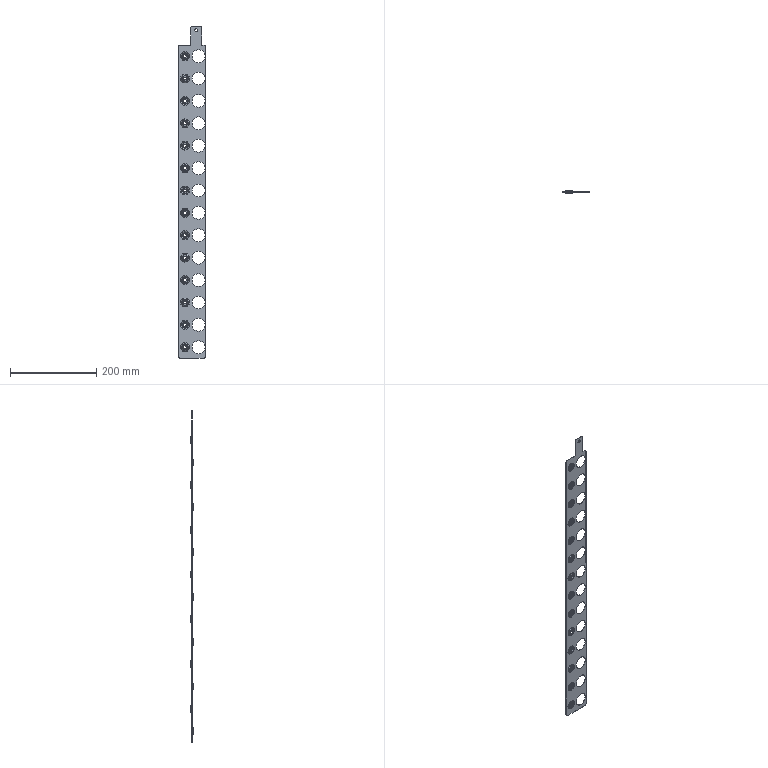Part | STEP file | 64524267 | 1 solid | 272 faces | box 64.7 x 6 x 771 mm | volume 38271 mm3 | torus 112 | cylinder 64 | cone 56 | plane 40 | commonest cylinder face diameters 7 x30 30 x28 8 x6